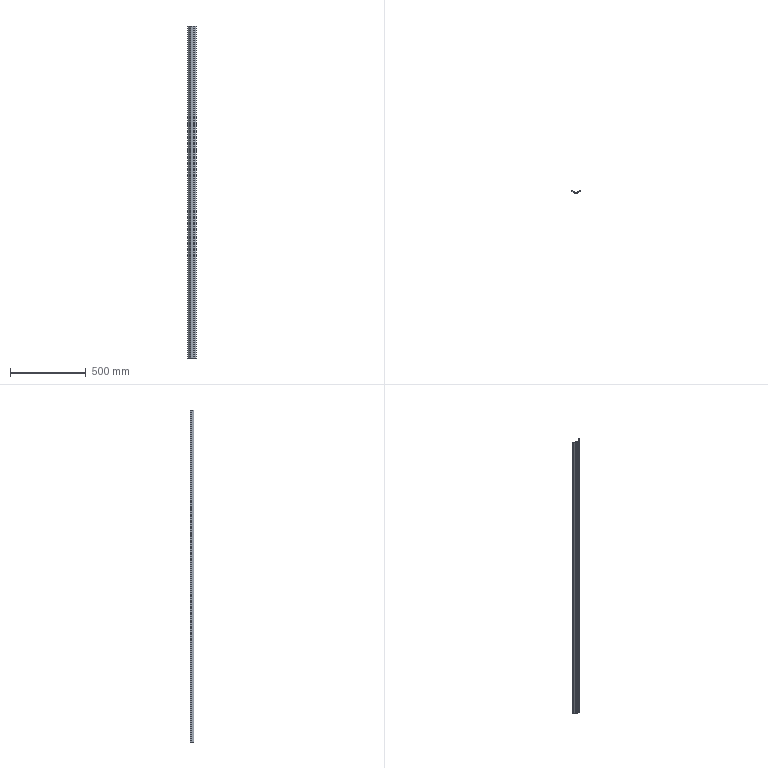Part | 1 solid | 40 faces | box 56.572 x 22.358 x 2185 mm | volume 366285 mm3 | plane 37 | cylinder 3 | commonest cylinder face diameters 1 x2 0.5 x1
STEP:
#1=CARTESIAN_POINT('',(6.75,2.,-1092.5));
#2=VERTEX_POINT('',#1);
#3=CARTESIAN_POINT('',(6.75,5.,-1092.5));
#4=VERTEX_POINT('',#3);
#5=CARTESIAN_POINT('',(6.75,2.,-1092.5));
#6=DIRECTION('',(0.,1.,0.));
#7=VECTOR('',#6,1000.);
#8=LINE('',#5,#7);
#9=EDGE_CURVE('',#2,#4,#8,.T.);
#10=ORIENTED_EDGE('',*,*,#9,.T.);
#11=CARTESIAN_POINT('',(6.75,5.,1092.5));
#12=VERTEX_POINT('',#11);
#13=CARTESIAN_POINT('',(6.75,5.,1092.5));
#14=DIRECTION('',(0.,0.,-1.));
#15=VECTOR('',#14,1000.);
#16=LINE('',#13,#15);
#17=EDGE_CURVE('',#12,#4,#16,.T.);
#18=ORIENTED_EDGE('',*,*,#17,.F.);
#19=CARTESIAN_POINT('',(6.75,2.,1092.5));
#20=VERTEX_POINT('',#19);
#21=CARTESIAN_POINT('',(6.75,2.,1092.5));
#22=DIRECTION('',(0.,1.,0.));
#23=VECTOR('',#22,1000.);
#24=LINE('',#21,#23);
#25=EDGE_CURVE('',#20,#12,#24,.T.);
#26=ORIENTED_EDGE('',*,*,#25,.F.);
#27=CARTESIAN_POINT('',(6.75,2.,1092.5));
#28=DIRECTION('',(0.,0.,-1.));
#29=VECTOR('',#28,1000.);
#30=LINE('',#27,#29);
#31=EDGE_CURVE('',#20,#2,#30,.T.);
#32=ORIENTED_EDGE('',*,*,#31,.T.);
#33=EDGE_LOOP('',(#10,#18,#26,#32));
#34=FACE_OUTER_BOUND('',#33,.T.);
#35=CARTESIAN_POINT('',(6.75,2.,1092.5));
#36=DIRECTION('',(-1.,0.,0.));
#37=DIRECTION('',(0.,0.,1.));
#38=AXIS2_PLACEMENT_3D('',#35,#36,#37);
#39=PLANE('',#38);
#40=ADVANCED_FACE('',(#34),#39,.F.);
#41=CARTESIAN_POINT('',(5.25,5.,-1092.5));
#42=VERTEX_POINT('',#41);
#43=CARTESIAN_POINT('',(6.75,5.,-1092.5));
#44=DIRECTION('',(-1.,0.,0.));
#45=VECTOR('',#44,1000.);
#46=LINE('',#43,#45);
#47=EDGE_CURVE('',#4,#42,#46,.T.);
#48=ORIENTED_EDGE('',*,*,#47,.T.);
#49=CARTESIAN_POINT('',(5.25,5.,1092.5));
#50=VERTEX_POINT('',#49);
#51=CARTESIAN_POINT('',(5.25,5.,1092.5));
#52=DIRECTION('',(0.,0.,-1.));
#53=VECTOR('',#52,1000.);
#54=LINE('',#51,#53);
#55=EDGE_CURVE('',#50,#42,#54,.T.);
#56=ORIENTED_EDGE('',*,*,#55,.F.);
#57=CARTESIAN_POINT('',(6.75,5.,1092.5));
#58=DIRECTION('',(-1.,0.,0.));
#59=VECTOR('',#58,1000.);
#60=LINE('',#57,#59);
#61=EDGE_CURVE('',#12,#50,#60,.T.);
#62=ORIENTED_EDGE('',*,*,#61,.F.);
#63=ORIENTED_EDGE('',*,*,#17,.T.);
#64=EDGE_LOOP('',(#48,#56,#62,#63));
#65=FACE_OUTER_BOUND('',#64,.T.);
#66=CARTESIAN_POINT('',(6.75,5.,1092.5));
#67=DIRECTION('',(0.,-1.,0.));
#68=DIRECTION('',(1.,0.,0.));
#69=AXIS2_PLACEMENT_3D('',#66,#67,#68);
#70=PLANE('',#69);
#71=ADVANCED_FACE('',(#65),#70,.F.);
#72=CARTESIAN_POINT('',(5.25,2.,-1092.5));
#73=VERTEX_POINT('',#72);
#74=CARTESIAN_POINT('',(5.25,5.,-1092.5));
#75=DIRECTION('',(0.,-1.,0.));
#76=VECTOR('',#75,1000.);
#77=LINE('',#74,#76);
#78=EDGE_CURVE('',#42,#73,#77,.T.);
#79=ORIENTED_EDGE('',*,*,#78,.T.);
#80=CARTESIAN_POINT('',(5.25,2.,1092.5));
#81=VERTEX_POINT('',#80);
#82=CARTESIAN_POINT('',(5.25,2.,1092.5));
#83=DIRECTION('',(0.,0.,-1.));
#84=VECTOR('',#83,1000.);
#85=LINE('',#82,#84);
#86=EDGE_CURVE('',#81,#73,#85,.T.);
#87=ORIENTED_EDGE('',*,*,#86,.F.);
#88=CARTESIAN_POINT('',(5.25,5.,1092.5));
#89=DIRECTION('',(0.,-1.,0.));
#90=VECTOR('',#89,1000.);
#91=LINE('',#88,#90);
#92=EDGE_CURVE('',#50,#81,#91,.T.);
#93=ORIENTED_EDGE('',*,*,#92,.F.);
#94=ORIENTED_EDGE('',*,*,#55,.T.);
#95=EDGE_LOOP('',(#79,#87,#93,#94));
#96=FACE_OUTER_BOUND('',#95,.T.);
#97=CARTESIAN_POINT('',(5.25,5.,1092.5));
#98=DIRECTION('',(1.,0.,0.));
#99=DIRECTION('',(0.,0.,-1.));
#100=AXIS2_PLACEMENT_3D('',#97,#98,#99);
#101=PLANE('',#100);
#102=ADVANCED_FACE('',(#96),#101,.F.);
#103=CARTESIAN_POINT('',(0.25,2.,-1092.5));
#104=VERTEX_POINT('',#103);
#105=CARTESIAN_POINT('',(5.25,2.,-1092.5));
#106=DIRECTION('',(-1.,0.,0.));
#107=VECTOR('',#106,1000.);
#108=LINE('',#105,#107);
#109=EDGE_CURVE('',#73,#104,#108,.T.);
#110=ORIENTED_EDGE('',*,*,#109,.T.);
#111=CARTESIAN_POINT('',(0.25,2.,1092.5));
#112=VERTEX_POINT('',#111);
#113=CARTESIAN_POINT('',(0.25,2.,1092.5));
#114=DIRECTION('',(0.,0.,-1.));
#115=VECTOR('',#114,1000.);
#116=LINE('',#113,#115);
#117=EDGE_CURVE('',#112,#104,#116,.T.);
#118=ORIENTED_EDGE('',*,*,#117,.F.);
#119=CARTESIAN_POINT('',(5.25,2.,1092.5));
#120=DIRECTION('',(-1.,0.,0.));
#121=VECTOR('',#120,1000.);
#122=LINE('',#119,#121);
#123=EDGE_CURVE('',#81,#112,#122,.T.);
#124=ORIENTED_EDGE('',*,*,#123,.F.);
#125=ORIENTED_EDGE('',*,*,#86,.T.);
#126=EDGE_LOOP('',(#110,#118,#124,#125));
#127=FACE_OUTER_BOUND('',#126,.T.);
#128=CARTESIAN_POINT('',(5.25,2.,1092.5));
#129=DIRECTION('',(0.,-1.,0.));
#130=DIRECTION('',(0.,0.,-1.));
#131=AXIS2_PLACEMENT_3D('',#128,#129,#130);
#132=PLANE('',#131);
#133=ADVANCED_FACE('',(#127),#132,.F.);
#134=CARTESIAN_POINT('',(-0.25,2.,-1092.5));
#135=VERTEX_POINT('',#134);
#136=CARTESIAN_POINT('',(0.,2.,-1092.5));
#137=DIRECTION('',(0.,0.,-1.));
#138=DIRECTION('',(1.,0.,0.));
#139=AXIS2_PLACEMENT_3D('',#136,#137,#138);
#140=CIRCLE('',#139,0.25);
#141=EDGE_CURVE('',#104,#135,#140,.T.);
#142=ORIENTED_EDGE('',*,*,#141,.T.);
#143=CARTESIAN_POINT('',(-0.25,2.,1092.5));
#144=VERTEX_POINT('',#143);
#145=CARTESIAN_POINT('',(-0.25,2.,1092.5));
#146=DIRECTION('',(0.,0.,-1.));
#147=VECTOR('',#146,1000.);
#148=LINE('',#145,#147);
#149=EDGE_CURVE('',#144,#135,#148,.T.);
#150=ORIENTED_EDGE('',*,*,#149,.F.);
#151=CARTESIAN_POINT('',(0.,2.,1092.5));
#152=DIRECTION('',(0.,0.,-1.));
#153=DIRECTION('',(1.,0.,0.));
#154=AXIS2_PLACEMENT_3D('',#151,#152,#153);
#155=CIRCLE('',#154,0.25);
#156=EDGE_CURVE('',#112,#144,#155,.T.);
#157=ORIENTED_EDGE('',*,*,#156,.F.);
#158=ORIENTED_EDGE('',*,*,#117,.T.);
#159=EDGE_LOOP('',(#142,#150,#157,#158));
#160=FACE_OUTER_BOUND('',#159,.T.);
#161=CARTESIAN_POINT('',(0.,2.,1092.5));
#162=DIRECTION('',(0.,0.,-1.));
#163=DIRECTION('',(-1.,0.,0.));
#164=AXIS2_PLACEMENT_3D('',#161,#162,#163);
#165=CYLINDRICAL_SURFACE('',#164,0.25);
#166=ADVANCED_FACE('',(#160),#165,.F.);
#167=CARTESIAN_POINT('',(-5.25,2.,-1092.5));
#168=VERTEX_POINT('',#167);
#169=CARTESIAN_POINT('',(-0.25,2.,-1092.5));
#170=DIRECTION('',(-1.,0.,0.));
#171=VECTOR('',#170,1000.);
#172=LINE('',#169,#171);
#173=EDGE_CURVE('',#135,#168,#172,.T.);
#174=ORIENTED_EDGE('',*,*,#173,.T.);
#175=CARTESIAN_POINT('',(-5.25,2.,1092.5));
#176=VERTEX_POINT('',#175);
#177=CARTESIAN_POINT('',(-5.25,2.,1092.5));
#178=DIRECTION('',(0.,0.,-1.));
#179=VECTOR('',#178,1000.);
#180=LINE('',#177,#179);
#181=EDGE_CURVE('',#176,#168,#180,.T.);
#182=ORIENTED_EDGE('',*,*,#181,.F.);
#183=CARTESIAN_POINT('',(-0.25,2.,1092.5));
#184=DIRECTION('',(-1.,0.,0.));
#185=VECTOR('',#184,1000.);
#186=LINE('',#183,#185);
#187=EDGE_CURVE('',#144,#176,#186,.T.);
#188=ORIENTED_EDGE('',*,*,#187,.F.);
#189=ORIENTED_EDGE('',*,*,#149,.T.);
#190=EDGE_LOOP('',(#174,#182,#188,#189));
#191=FACE_OUTER_BOUND('',#190,.T.);
#192=CARTESIAN_POINT('',(-0.25,2.,1092.5));
#193=DIRECTION('',(0.,-1.,0.));
#194=DIRECTION('',(1.,0.,0.));
#195=AXIS2_PLACEMENT_3D('',#192,#193,#194);
#196=PLANE('',#195);
#197=ADVANCED_FACE('',(#191),#196,.F.);
#198=CARTESIAN_POINT('',(-5.25,5.,-1092.5));
#199=VERTEX_POINT('',#198);
#200=CARTESIAN_POINT('',(-5.25,2.,-1092.5));
#201=DIRECTION('',(0.,1.,0.));
#202=VECTOR('',#201,1000.);
#203=LINE('',#200,#202);
#204=EDGE_CURVE('',#168,#199,#203,.T.);
#205=ORIENTED_EDGE('',*,*,#204,.T.);
#206=CARTESIAN_POINT('',(-5.25,5.,1092.5));
#207=VERTEX_POINT('',#206);
#208=CARTESIAN_POINT('',(-5.25,5.,1092.5));
#209=DIRECTION('',(0.,0.,-1.));
#210=VECTOR('',#209,1000.);
#211=LINE('',#208,#210);
#212=EDGE_CURVE('',#207,#199,#211,.T.);
#213=ORIENTED_EDGE('',*,*,#212,.F.);
#214=CARTESIAN_POINT('',(-5.25,2.,1092.5));
#215=DIRECTION('',(0.,1.,0.));
#216=VECTOR('',#215,1000.);
#217=LINE('',#214,#216);
#218=EDGE_CURVE('',#176,#207,#217,.T.);
#219=ORIENTED_EDGE('',*,*,#218,.F.);
#220=ORIENTED_EDGE('',*,*,#181,.T.);
#221=EDGE_LOOP('',(#205,#213,#219,#220));
#222=FACE_OUTER_BOUND('',#221,.T.);
#223=CARTESIAN_POINT('',(-5.25,2.,1092.5));
#224=DIRECTION('',(-1.,0.,0.));
#225=DIRECTION('',(0.,0.,1.));
#226=AXIS2_PLACEMENT_3D('',#223,#224,#225);
#227=PLANE('',#226);
#228=ADVANCED_FACE('',(#222),#227,.F.);
#229=CARTESIAN_POINT('',(-6.75,5.,-1092.5));
#230=VERTEX_POINT('',#229);
#231=CARTESIAN_POINT('',(-5.25,5.,-1092.5));
#232=DIRECTION('',(-1.,0.,0.));
#233=VECTOR('',#232,1000.);
#234=LINE('',#231,#233);
#235=EDGE_CURVE('',#199,#230,#234,.T.);
#236=ORIENTED_EDGE('',*,*,#235,.T.);
#237=CARTESIAN_POINT('',(-6.75,5.,1092.5));
#238=VERTEX_POINT('',#237);
#239=CARTESIAN_POINT('',(-6.75,5.,1092.5));
#240=DIRECTION('',(0.,0.,-1.));
#241=VECTOR('',#240,1000.);
#242=LINE('',#239,#241);
#243=EDGE_CURVE('',#238,#230,#242,.T.);
#244=ORIENTED_EDGE('',*,*,#243,.F.);
#245=CARTESIAN_POINT('',(-5.25,5.,1092.5));
#246=DIRECTION('',(-1.,0.,0.));
#247=VECTOR('',#246,1000.);
#248=LINE('',#245,#247);
#249=EDGE_CURVE('',#207,#238,#248,.T.);
#250=ORIENTED_EDGE('',*,*,#249,.F.);
#251=ORIENTED_EDGE('',*,*,#212,.T.);
#252=EDGE_LOOP('',(#236,#244,#250,#251));
#253=FACE_OUTER_BOUND('',#252,.T.);
#254=CARTESIAN_POINT('',(-5.25,5.,1092.5));
#255=DIRECTION('',(0.,-1.,0.));
#256=DIRECTION('',(1.,0.,0.));
#257=AXIS2_PLACEMENT_3D('',#254,#255,#256);
#258=PLANE('',#257);
#259=ADVANCED_FACE('',(#253),#258,.F.);
#260=CARTESIAN_POINT('',(-6.75,2.,-1092.5));
#261=VERTEX_POINT('',#260);
#262=CARTESIAN_POINT('',(-6.75,5.,-1092.5));
#263=DIRECTION('',(0.,-1.,0.));
#264=VECTOR('',#263,1000.);
#265=LINE('',#262,#264);
#266=EDGE_CURVE('',#230,#261,#265,.T.);
#267=ORIENTED_EDGE('',*,*,#266,.T.);
#268=CARTESIAN_POINT('',(-6.75,2.,1092.5));
#269=VERTEX_POINT('',#268);
#270=CARTESIAN_POINT('',(-6.75,2.,1092.5));
#271=DIRECTION('',(0.,0.,-1.));
#272=VECTOR('',#271,1000.);
#273=LINE('',#270,#272);
#274=EDGE_CURVE('',#269,#261,#273,.T.);
#275=ORIENTED_EDGE('',*,*,#274,.F.);
#276=CARTESIAN_POINT('',(-6.75,5.,1092.5));
#277=DIRECTION('',(0.,-1.,0.));
#278=VECTOR('',#277,1000.);
#279=LINE('',#276,#278);
#280=EDGE_CURVE('',#238,#269,#279,.T.);
#281=ORIENTED_EDGE('',*,*,#280,.F.);
#282=ORIENTED_EDGE('',*,*,#243,.T.);
#283=EDGE_LOOP('',(#267,#275,#281,#282));
#284=FACE_OUTER_BOUND('',#283,.T.);
#285=CARTESIAN_POINT('',(-6.75,5.,1092.5));
#286=DIRECTION('',(1.,0.,0.));
#287=DIRECTION('',(0.,0.,-1.));
#288=AXIS2_PLACEMENT_3D('',#285,#286,#287);
#289=PLANE('',#288);
#290=ADVANCED_FACE('',(#284),#289,.F.);
#291=CARTESIAN_POINT('',(-8.635,2.,-1092.5));
#292=VERTEX_POINT('',#291);
#293=CARTESIAN_POINT('',(-6.75,2.,-1092.5));
#294=DIRECTION('',(-1.,0.,0.));
#295=VECTOR('',#294,1000.);
#296=LINE('',#293,#295);
#297=EDGE_CURVE('',#261,#292,#296,.T.);
#298=ORIENTED_EDGE('',*,*,#297,.T.);
#299=CARTESIAN_POINT('',(-8.635,2.,1092.5));
#300=VERTEX_POINT('',#299);
#301=CARTESIAN_POINT('',(-8.635,2.,1092.5));
#302=DIRECTION('',(0.,0.,-1.));
#303=VECTOR('',#302,1000.);
#304=LINE('',#301,#303);
#305=EDGE_CURVE('',#300,#292,#304,.T.);
#306=ORIENTED_EDGE('',*,*,#305,.F.);
#307=CARTESIAN_POINT('',(-6.75,2.,1092.5));
#308=DIRECTION('',(-1.,0.,0.));
#309=VECTOR('',#308,1000.);
#310=LINE('',#307,#309);
#311=EDGE_CURVE('',#269,#300,#310,.T.);
#312=ORIENTED_EDGE('',*,*,#311,.F.);
#313=ORIENTED_EDGE('',*,*,#274,.T.);
#314=EDGE_LOOP('',(#298,#306,#312,#313));
#315=FACE_OUTER_BOUND('',#314,.T.);
#316=CARTESIAN_POINT('',(-6.75,2.,1092.5));
#317=DIRECTION('',(0.,-1.,0.));
#318=DIRECTION('',(1.,0.,0.));
#319=AXIS2_PLACEMENT_3D('',#316,#317,#318);
#320=PLANE('',#319);
#321=ADVANCED_FACE('',(#315),#320,.F.);
#322=CARTESIAN_POINT('',(-11.75,5.119,-1092.5));
#323=VERTEX_POINT('',#322);
#324=CARTESIAN_POINT('',(-8.635,2.,-1092.5));
#325=DIRECTION('',(-0.7067,0.7076,0.));
#326=VECTOR('',#325,1000.);
#327=LINE('',#324,#326);
#328=EDGE_CURVE('',#292,#323,#327,.T.);
#329=ORIENTED_EDGE('',*,*,#328,.T.);
#330=CARTESIAN_POINT('',(-11.75,5.119,1092.5));
#331=VERTEX_POINT('',#330);
#332=CARTESIAN_POINT('',(-11.75,5.119,1092.5));
#333=DIRECTION('',(0.,0.,-1.));
#334=VECTOR('',#333,1000.);
#335=LINE('',#332,#334);
#336=EDGE_CURVE('',#331,#323,#335,.T.);
#337=ORIENTED_EDGE('',*,*,#336,.F.);
#338=CARTESIAN_POINT('',(-8.635,2.,1092.5));
#339=DIRECTION('',(-0.7067,0.7076,0.));
#340=VECTOR('',#339,1000.);
#341=LINE('',#338,#340);
#342=EDGE_CURVE('',#300,#331,#341,.T.);
#343=ORIENTED_EDGE('',*,*,#342,.F.);
#344=ORIENTED_EDGE('',*,*,#305,.T.);
#345=EDGE_LOOP('',(#329,#337,#343,#344));
#346=FACE_OUTER_BOUND('',#345,.T.);
#347=CARTESIAN_POINT('',(-8.635,2.,1092.5));
#348=DIRECTION('',(-0.7076,-0.7067,0.));
#349=DIRECTION('',(0.7067,-0.7076,0.));
#350=AXIS2_PLACEMENT_3D('',#347,#348,#349);
#351=PLANE('',#350);
#352=ADVANCED_FACE('',(#346),#351,.F.);
#353=CARTESIAN_POINT('',(-11.75,8.887,-1092.5));
#354=VERTEX_POINT('',#353);
#355=CARTESIAN_POINT('',(-11.75,5.119,-1092.5));
#356=DIRECTION('',(0.,1.,0.));
#357=VECTOR('',#356,1000.);
#358=LINE('',#355,#357);
#359=EDGE_CURVE('',#323,#354,#358,.T.);
#360=ORIENTED_EDGE('',*,*,#359,.T.);
#361=CARTESIAN_POINT('',(-11.75,8.887,1092.5));
#362=VERTEX_POINT('',#361);
#363=CARTESIAN_POINT('',(-11.75,8.887,1092.5));
#364=DIRECTION('',(0.,0.,-1.));
#365=VECTOR('',#364,1000.);
#366=LINE('',#363,#365);
#367=EDGE_CURVE('',#362,#354,#366,.T.);
#368=ORIENTED_EDGE('',*,*,#367,.F.);
#369=CARTESIAN_POINT('',(-11.75,5.119,1092.5));
#370=DIRECTION('',(0.,1.,0.));
#371=VECTOR('',#370,1000.);
#372=LINE('',#369,#371);
#373=EDGE_CURVE('',#331,#362,#372,.T.);
#374=ORIENTED_EDGE('',*,*,#373,.F.);
#375=ORIENTED_EDGE('',*,*,#336,.T.);
#376=EDGE_LOOP('',(#360,#368,#374,#375));
#377=FACE_OUTER_BOUND('',#376,.T.);
#378=CARTESIAN_POINT('',(-11.75,5.119,1092.5));
#379=DIRECTION('',(-1.,0.,0.));
#380=DIRECTION('',(0.,0.,1.));
#381=AXIS2_PLACEMENT_3D('',#378,#379,#380);
#382=PLANE('',#381);
#383=ADVANCED_FACE('',(#377),#382,.F.);
#384=CARTESIAN_POINT('',(-12.25,9.387,-1092.5));
#385=VERTEX_POINT('',#384);
#386=CARTESIAN_POINT('',(-11.75,8.887,-1092.5));
#387=DIRECTION('',(-0.7071,0.7071,0.));
#388=VECTOR('',#387,1000.);
#389=LINE('',#386,#388);
#390=EDGE_CURVE('',#354,#385,#389,.T.);
#391=ORIENTED_EDGE('',*,*,#390,.T.);
#392=CARTESIAN_POINT('',(-12.25,9.387,1092.5));
#393=VERTEX_POINT('',#392);
#394=CARTESIAN_POINT('',(-12.25,9.387,1092.5));
#395=DIRECTION('',(0.,0.,-1.));
#396=VECTOR('',#395,1000.);
#397=LINE('',#394,#396);
#398=EDGE_CURVE('',#393,#385,#397,.T.);
#399=ORIENTED_EDGE('',*,*,#398,.F.);
#400=CARTESIAN_POINT('',(-11.75,8.887,1092.5));
#401=DIRECTION('',(-0.7071,0.7071,0.));
#402=VECTOR('',#401,1000.);
#403=LINE('',#400,#402);
#404=EDGE_CURVE('',#362,#393,#403,.T.);
#405=ORIENTED_EDGE('',*,*,#404,.F.);
#406=ORIENTED_EDGE('',*,*,#367,.T.);
#407=EDGE_LOOP('',(#391,#399,#405,#406));
#408=FACE_OUTER_BOUND('',#407,.T.);
#409=CARTESIAN_POINT('',(-11.75,8.887,1092.5));
#410=DIRECTION('',(-0.7071,-0.7071,0.));
#411=DIRECTION('',(0.7071,-0.7071,0.));
#412=AXIS2_PLACEMENT_3D('',#409,#410,#411);
#413=PLANE('',#412);
#414=ADVANCED_FACE('',(#408),#413,.F.);
#415=CARTESIAN_POINT('',(-12.75,9.387,-1092.5));
#416=VERTEX_POINT('',#415);
#417=CARTESIAN_POINT('',(-12.25,9.387,-1092.5));
#418=DIRECTION('',(-1.,0.,0.));
#419=VECTOR('',#418,1000.);
#420=LINE('',#417,#419);
#421=EDGE_CURVE('',#385,#416,#420,.T.);
#422=ORIENTED_EDGE('',*,*,#421,.T.);
#423=CARTESIAN_POINT('',(-12.75,9.387,1092.5));
#424=VERTEX_POINT('',#423);
#425=CARTESIAN_POINT('',(-12.75,9.387,1092.5));
#426=DIRECTION('',(0.,0.,-1.));
#427=VECTOR('',#426,1000.);
#428=LINE('',#425,#427);
#429=EDGE_CURVE('',#424,#416,#428,.T.);
#430=ORIENTED_EDGE('',*,*,#429,.F.);
#431=CARTESIAN_POINT('',(-12.25,9.387,1092.5));
#432=DIRECTION('',(-1.,0.,0.));
#433=VECTOR('',#432,1000.);
#434=LINE('',#431,#433);
#435=EDGE_CURVE('',#393,#424,#434,.T.);
#436=ORIENTED_EDGE('',*,*,#435,.F.);
#437=ORIENTED_EDGE('',*,*,#398,.T.);
#438=EDGE_LOOP('',(#422,#430,#436,#437));
#439=FACE_OUTER_BOUND('',#438,.T.);
#440=CARTESIAN_POINT('',(-12.25,9.387,1092.5));
#441=DIRECTION('',(0.,-1.,0.));
#442=DIRECTION('',(0.,0.,-1.));
#443=AXIS2_PLACEMENT_3D('',#440,#441,#442);
#444=PLANE('',#443);
#445=ADVANCED_FACE('',(#439),#444,.F.);
#446=CARTESIAN_POINT('',(-12.75,7.328,-1092.5));
#447=VERTEX_POINT('',#446);
#448=CARTESIAN_POINT('',(-12.75,9.387,-1092.5));
#449=DIRECTION('',(0.,-1.,0.));
#450=VECTOR('',#449,1000.);
#451=LINE('',#448,#450);
#452=EDGE_CURVE('',#416,#447,#451,.T.);
#453=ORIENTED_EDGE('',*,*,#452,.T.);
#454=CARTESIAN_POINT('',(-12.75,7.328,1092.5));
#455=VERTEX_POINT('',#454);
#456=CARTESIAN_POINT('',(-12.75,7.328,1092.5));
#457=DIRECTION('',(0.,0.,-1.));
#458=VECTOR('',#457,1000.);
#459=LINE('',#456,#458);
#460=EDGE_CURVE('',#455,#447,#459,.T.);
#461=ORIENTED_EDGE('',*,*,#460,.F.);
#462=CARTESIAN_POINT('',(-12.75,9.387,1092.5));
#463=DIRECTION('',(0.,-1.,0.));
#464=VECTOR('',#463,1000.);
#465=LINE('',#462,#464);
#466=EDGE_CURVE('',#424,#455,#465,.T.);
#467=ORIENTED_EDGE('',*,*,#466,.F.);
#468=ORIENTED_EDGE('',*,*,#429,.T.);
#469=EDGE_LOOP('',(#453,#461,#467,#468));
#470=FACE_OUTER_BOUND('',#469,.T.);
#471=CARTESIAN_POINT('',(-12.75,9.387,1092.5));
#472=DIRECTION('',(1.,0.,0.));
#473=DIRECTION('',(0.,0.,-1.));
#474=AXIS2_PLACEMENT_3D('',#471,#472,#473);
#475=PLANE('',#474);
#476=ADVANCED_FACE('',(#470),#475,.F.);
#477=CARTESIAN_POINT('',(-13.604,6.975,-1092.5));
#478=VERTEX_POINT('',#477);
#479=CARTESIAN_POINT('',(-13.25,7.328,-1092.5));
#480=DIRECTION('',(0.,0.,-1.));
#481=DIRECTION('',(1.,0.,0.));
#482=AXIS2_PLACEMENT_3D('',#479,#480,#481);
#483=CIRCLE('',#482,0.5);
#484=EDGE_CURVE('',#447,#478,#483,.T.);
#485=ORIENTED_EDGE('',*,*,#484,.T.);
#486=CARTESIAN_POINT('',(-13.604,6.975,1092.5));
#487=VERTEX_POINT('',#486);
#488=CARTESIAN_POINT('',(-13.604,6.975,1092.5));
#489=DIRECTION('',(0.,0.,-1.));
#490=VECTOR('',#489,1000.);
#491=LINE('',#488,#490);
#492=EDGE_CURVE('',#487,#478,#491,.T.);
#493=ORIENTED_EDGE('',*,*,#492,.F.);
#494=CARTESIAN_POINT('',(-13.25,7.328,1092.5));
#495=DIRECTION('',(0.,0.,-1.));
#496=DIRECTION('',(1.,0.,0.));
#497=AXIS2_PLACEMENT_3D('',#494,#495,#496);
#498=CIRCLE('',#497,0.5);
#499=EDGE_CURVE('',#455,#487,#498,.T.);
#500=ORIENTED_EDGE('',*,*,#499,.F.);
#501=ORIENTED_EDGE('',*,*,#460,.T.);
#502=EDGE_LOOP('',(#485,#493,#500,#501));
#503=FACE_OUTER_BOUND('',#502,.T.);
#504=CARTESIAN_POINT('',(-13.25,7.328,1092.5));
#505=DIRECTION('',(0.,0.,-1.));
#506=DIRECTION('',(-1.,0.,0.));
#507=AXIS2_PLACEMENT_3D('',#504,#505,#506);
#508=CYLINDRICAL_SURFACE('',#507,0.5);
#509=ADVANCED_FACE('',(#503),#508,.F.);
#510=CARTESIAN_POINT('',(-23.891,17.282,-1092.5));
#511=VERTEX_POINT('',#510);
#512=CARTESIAN_POINT('',(-13.604,6.975,-1092.5));
#513=DIRECTION('',(-0.7064,0.7078,0.));
#514=VECTOR('',#513,1000.);
#515=LINE('',#512,#514);
#516=EDGE_CURVE('',#478,#511,#515,.T.);
#517=ORIENTED_EDGE('',*,*,#516,.T.);
#518=CARTESIAN_POINT('',(-23.891,17.282,1092.5));
#519=VERTEX_POINT('',#518);
#520=CARTESIAN_POINT('',(-23.891,17.282,1092.5));
#521=DIRECTION('',(0.,0.,-1.));
#522=VECTOR('',#521,1000.);
#523=LINE('',#520,#522);
#524=EDGE_CURVE('',#519,#511,#523,.T.);
#525=ORIENTED_EDGE('',*,*,#524,.F.);
#526=CARTESIAN_POINT('',(-13.604,6.975,1092.5));
#527=DIRECTION('',(-0.7064,0.7078,0.));
#528=VECTOR('',#527,1000.);
#529=LINE('',#526,#528);
#530=EDGE_CURVE('',#487,#519,#529,.T.);
#531=ORIENTED_EDGE('',*,*,#530,.F.);
#532=ORIENTED_EDGE('',*,*,#492,.T.);
#533=EDGE_LOOP('',(#517,#525,#531,#532));
#534=FACE_OUTER_BOUND('',#533,.T.);
#535=CARTESIAN_POINT('',(-13.604,6.975,1092.5));
#536=DIRECTION('',(-0.7078,-0.7064,0.));
#537=DIRECTION('',(0.7064,-0.7078,0.));
#538=AXIS2_PLACEMENT_3D('',#535,#536,#537);
#539=PLANE('',#538);
#540=ADVANCED_FACE('',(#534),#539,.F.);
#541=CARTESIAN_POINT('',(-23.891,19.376,-1092.5));
#542=VERTEX_POINT('',#541);
#543=CARTESIAN_POINT('',(-23.891,17.282,-1092.5));
#544=DIRECTION('',(0.,1.,0.));
#545=VECTOR('',#544,1000.);
#546=LINE('',#543,#545);
#547=EDGE_CURVE('',#511,#542,#546,.T.);
#548=ORIENTED_EDGE('',*,*,#547,.T.);
#549=CARTESIAN_POINT('',(-23.891,19.376,1092.5));
#550=VERTEX_POINT('',#549);
#551=CARTESIAN_POINT('',(-23.891,19.376,1092.5));
#552=DIRECTION('',(0.,0.,-1.));
#553=VECTOR('',#552,1000.);
#554=LINE('',#551,#553);
#555=EDGE_CURVE('',#550,#542,#554,.T.);
#556=ORIENTED_EDGE('',*,*,#555,.F.);
#557=CARTESIAN_POINT('',(-23.891,17.282,1092.5));
#558=DIRECTION('',(0.,1.,0.));
#559=VECTOR('',#558,1000.);
#560=LINE('',#557,#559);
#561=EDGE_CURVE('',#519,#550,#560,.T.);
#562=ORIENTED_EDGE('',*,*,#561,.F.);
#563=ORIENTED_EDGE('',*,*,#524,.T.);
#564=EDGE_LOOP('',(#548,#556,#562,#563));
#565=FACE_OUTER_BOUND('',#564,.T.);
#566=CARTESIAN_POINT('',(-23.891,17.282,1092.5));
#567=DIRECTION('',(-1.,0.,0.));
#568=DIRECTION('',(0.,0.,1.));
#569=AXIS2_PLACEMENT_3D('',#566,#567,#568);
#570=PLANE('',#569);
#571=ADVANCED_FACE('',(#565),#570,.F.);
#572=CARTESIAN_POINT('',(-26.873,22.358,-1092.5));
#573=VERTEX_POINT('',#572);
#574=CARTESIAN_POINT('',(-23.891,19.376,-1092.5));
#575=DIRECTION('',(-0.7071,0.7071,0.));
#576=VECTOR('',#575,1000.);
#577=LINE('',#574,#576);
#578=EDGE_CURVE('',#542,#573,#577,.T.);
#579=ORIENTED_EDGE('',*,*,#578,.T.);
#580=CARTESIAN_POINT('',(-26.873,22.358,1092.5));
#581=VERTEX_POINT('',#580);
#582=CARTESIAN_POINT('',(-26.873,22.358,1092.5));
#583=DIRECTION('',(0.,0.,-1.));
#584=VECTOR('',#583,1000.);
#585=LINE('',#582,#584);
#586=EDGE_CURVE('',#581,#573,#585,.T.);
#587=ORIENTED_EDGE('',*,*,#586,.F.);
#588=CARTESIAN_POINT('',(-23.891,19.376,1092.5));
#589=DIRECTION('',(-0.7071,0.7071,0.));
#590=VECTOR('',#589,1000.);
#591=LINE('',#588,#590);
#592=EDGE_CURVE('',#550,#581,#591,.T.);
#593=ORIENTED_EDGE('',*,*,#592,.F.);
#594=ORIENTED_EDGE('',*,*,#555,.T.);
#595=EDGE_LOOP('',(#579,#587,#593,#594));
#596=FACE_OUTER_BOUND('',#595,.T.);
#597=CARTESIAN_POINT('',(-23.891,19.376,1092.5));
#598=DIRECTION('',(-0.7071,-0.7071,0.));
#599=DIRECTION('',(0.7071,-0.7071,0.));
#600=AXIS2_PLACEMENT_3D('',#597,#598,#599);
#601=PLANE('',#600);
#602=ADVANCED_FACE('',(#596),#601,.F.);
#603=CARTESIAN_POINT('',(-27.58,22.358,-1092.5));
#604=VERTEX_POINT('',#603);
#605=CARTESIAN_POINT('',(-26.873,22.358,-1092.5));
#606=DIRECTION('',(-1.,0.,0.));
#607=VECTOR('',#606,1000.);
#608=LINE('',#605,#607);
#609=EDGE_CURVE('',#573,#604,#608,.T.);
#610=ORIENTED_EDGE('',*,*,#609,.T.);
#611=CARTESIAN_POINT('',(-27.58,22.358,1092.5));
#612=VERTEX_POINT('',#611);
#613=CARTESIAN_POINT('',(-27.58,22.358,1092.5));
#614=DIRECTION('',(0.,0.,-1.));
#615=VECTOR('',#614,1000.);
#616=LINE('',#613,#615);
#617=EDGE_CURVE('',#612,#604,#616,.T.);
#618=ORIENTED_EDGE('',*,*,#617,.F.);
#619=CARTESIAN_POINT('',(-26.873,22.358,1092.5));
#620=DIRECTION('',(-1.,0.,0.));
#621=VECTOR('',#620,1000.);
#622=LINE('',#619,#621);
#623=EDGE_CURVE('',#581,#612,#622,.T.);
#624=ORIENTED_EDGE('',*,*,#623,.F.);
#625=ORIENTED_EDGE('',*,*,#586,.T.);
#626=EDGE_LOOP('',(#610,#618,#624,#625));
#627=FACE_OUTER_BOUND('',#626,.T.);
#628=CARTESIAN_POINT('',(-26.873,22.358,1092.5));
#629=DIRECTION('',(0.,-1.,0.));
#630=DIRECTION('',(0.,0.,-1.));
#631=AXIS2_PLACEMENT_3D('',#628,#629,#630);
#632=PLANE('',#631);
#633=ADVANCED_FACE('',(#627),#632,.F.);
#634=CARTESIAN_POINT('',(-28.284,21.654,-1092.5));
#635=VERTEX_POINT('',#634);
#636=CARTESIAN_POINT('',(-27.58,22.358,-1092.5));
#637=DIRECTION('',(-0.7071,-0.7071,0.));
#638=VECTOR('',#637,1000.);
#639=LINE('',#636,#638);
#640=EDGE_CURVE('',#604,#635,#639,.T.);
#641=ORIENTED_EDGE('',*,*,#640,.T.);
#642=CARTESIAN_POINT('',(-28.284,21.654,1092.5));
#643=VERTEX_POINT('',#642);
#644=CARTESIAN_POINT('',(-28.284,21.654,1092.5));
#645=DIRECTION('',(0.,0.,-1.));
#646=VECTOR('',#645,1000.);
#647=LINE('',#644,#646);
#648=EDGE_CURVE('',#643,#635,#647,.T.);
#649=ORIENTED_EDGE('',*,*,#648,.F.);
#650=CARTESIAN_POINT('',(-27.58,22.358,1092.5));
#651=DIRECTION('',(-0.7071,-0.7071,0.));
#652=VECTOR('',#651,1000.);
#653=LINE('',#650,#652);
#654=EDGE_CURVE('',#612,#643,#653,.T.);
#655=ORIENTED_EDGE('',*,*,#654,.F.);
#656=ORIENTED_EDGE('',*,*,#617,.T.);
#657=EDGE_LOOP('',(#641,#649,#655,#656));
#658=FACE_OUTER_BOUND('',#657,.T.);
#659=CARTESIAN_POINT('',(-27.58,22.358,1092.5));
#660=DIRECTION('',(0.7071,-0.7071,0.));
#661=DIRECTION('',(0.7071,0.7071,0.));
#662=AXIS2_PLACEMENT_3D('',#659,#660,#661);
#663=PLANE('',#662);
#664=ADVANCED_FACE('',(#658),#663,.F.);
#665=CARTESIAN_POINT('',(-28.284,19.103,-1092.5));
#666=VERTEX_POINT('',#665);
#667=CARTESIAN_POINT('',(-28.284,21.654,-1092.5));
#668=DIRECTION('',(0.,-1.,0.));
#669=VECTOR('',#668,1000.);
#670=LINE('',#667,#669);
#671=EDGE_CURVE('',#635,#666,#670,.T.);
#672=ORIENTED_EDGE('',*,*,#671,.T.);
#673=CARTESIAN_POINT('',(-28.284,19.103,1092.5));
#674=VERTEX_POINT('',#673);
#675=CARTESIAN_POINT('',(-28.284,19.103,1092.5));
#676=DIRECTION('',(0.,0.,-1.));
#677=VECTOR('',#676,1000.);
#678=LINE('',#675,#677);
#679=EDGE_CURVE('',#674,#666,#678,.T.);
#680=ORIENTED_EDGE('',*,*,#679,.F.);
#681=CARTESIAN_POINT('',(-28.284,21.654,1092.5));
#682=DIRECTION('',(0.,-1.,0.));
#683=VECTOR('',#682,1000.);
#684=LINE('',#681,#683);
#685=EDGE_CURVE('',#643,#674,#684,.T.);
#686=ORIENTED_EDGE('',*,*,#685,.F.);
#687=ORIENTED_EDGE('',*,*,#648,.T.);
#688=EDGE_LOOP('',(#672,#680,#686,#687));
#689=FACE_OUTER_BOUND('',#688,.T.);
#690=CARTESIAN_POINT('',(-28.284,21.654,1092.5));
#691=DIRECTION('',(1.,0.,0.));
#692=DIRECTION('',(0.,0.,-1.));
#693=AXIS2_PLACEMENT_3D('',#690,#691,#692);
#694=PLANE('',#693);
#695=ADVANCED_FACE('',(#689),#694,.F.);
#696=CARTESIAN_POINT('',(-9.182,0.,-1092.5));
#697=VERTEX_POINT('',#696);
#698=CARTESIAN_POINT('',(-28.284,19.103,-1092.5));
#699=DIRECTION('',(0.7071,-0.7071,0.));
#700=VECTOR('',#699,1000.);
#701=LINE('',#698,#700);
#702=EDGE_CURVE('',#666,#697,#701,.T.);
#703=ORIENTED_EDGE('',*,*,#702,.T.);
#704=CARTESIAN_POINT('',(-9.182,0.,1092.5));
#705=VERTEX_POINT('',#704);
#706=CARTESIAN_POINT('',(-9.182,0.,1092.5));
#707=DIRECTION('',(0.,0.,-1.));
#708=VECTOR('',#707,1000.);
#709=LINE('',#706,#708);
#710=EDGE_CURVE('',#705,#697,#709,.T.);
#711=ORIENTED_EDGE('',*,*,#710,.F.);
#712=CARTESIAN_POINT('',(-28.284,19.103,1092.5));
#713=DIRECTION('',(0.7071,-0.7071,0.));
#714=VECTOR('',#713,1000.);
#715=LINE('',#712,#714);
#716=EDGE_CURVE('',#674,#705,#715,.T.);
#717=ORIENTED_EDGE('',*,*,#716,.F.);
#718=ORIENTED_EDGE('',*,*,#679,.T.);
#719=EDGE_LOOP('',(#703,#711,#717,#718));
#720=FACE_OUTER_BOUND('',#719,.T.);
#721=CARTESIAN_POINT('',(-28.284,19.103,1092.5));
#722=DIRECTION('',(0.7071,0.7071,0.));
#723=DIRECTION('',(-0.7071,0.7071,0.));
#724=AXIS2_PLACEMENT_3D('',#721,#722,#723);
#725=PLANE('',#724);
#726=ADVANCED_FACE('',(#720),#725,.F.);
#727=CARTESIAN_POINT('',(9.182,0.,-1092.5));
#728=VERTEX_POINT('',#727);
#729=CARTESIAN_POINT('',(-9.182,0.,-1092.5));
#730=DIRECTION('',(1.,0.,0.));
#731=VECTOR('',#730,1000.);
#732=LINE('',#729,#731);
#733=EDGE_CURVE('',#697,#728,#732,.T.);
#734=ORIENTED_EDGE('',*,*,#733,.T.);
#735=CARTESIAN_POINT('',(9.182,0.,1092.5));
#736=VERTEX_POINT('',#735);
#737=CARTESIAN_POINT('',(9.182,0.,1092.5));
#738=DIRECTION('',(0.,0.,-1.));
#739=VECTOR('',#738,1000.);
#740=LINE('',#737,#739);
#741=EDGE_CURVE('',#736,#728,#740,.T.);
#742=ORIENTED_EDGE('',*,*,#741,.F.);
#743=CARTESIAN_POINT('',(-9.182,0.,1092.5));
#744=DIRECTION('',(1.,0.,0.));
#745=VECTOR('',#744,1000.);
#746=LINE('',#743,#745);
#747=EDGE_CURVE('',#705,#736,#746,.T.);
#748=ORIENTED_EDGE('',*,*,#747,.F.);
#749=ORIENTED_EDGE('',*,*,#710,.T.);
#750=EDGE_LOOP('',(#734,#742,#748,#749));
#751=FACE_OUTER_BOUND('',#750,.T.);
#752=CARTESIAN_POINT('',(-9.182,0.,1092.5));
#753=DIRECTION('',(0.,1.,0.));
#754=DIRECTION('',(-1.,0.,0.));
#755=AXIS2_PLACEMENT_3D('',#752,#753,#754);
#756=PLANE('',#755);
#757=ADVANCED_FACE('',(#751),#756,.F.);
#758=CARTESIAN_POINT('',(28.287,19.106,-1092.5));
#759=VERTEX_POINT('',#758);
#760=CARTESIAN_POINT('',(9.182,0.,-1092.5));
#761=DIRECTION('',(0.7071,0.7071,0.));
#762=VECTOR('',#761,1000.);
#763=LINE('',#760,#762);
#764=EDGE_CURVE('',#728,#759,#763,.T.);
#765=ORIENTED_EDGE('',*,*,#764,.T.);
#766=CARTESIAN_POINT('',(28.287,19.106,1092.5));
#767=VERTEX_POINT('',#766);
#768=CARTESIAN_POINT('',(28.287,19.106,1092.5));
#769=DIRECTION('',(0.,0.,-1.));
#770=VECTOR('',#769,1000.);
#771=LINE('',#768,#770);
#772=EDGE_CURVE('',#767,#759,#771,.T.);
#773=ORIENTED_EDGE('',*,*,#772,.F.);
#774=CARTESIAN_POINT('',(9.182,0.,1092.5));
#775=DIRECTION('',(0.7071,0.7071,0.));
#776=VECTOR('',#775,1000.);
#777=LINE('',#774,#776);
#778=EDGE_CURVE('',#736,#767,#777,.T.);
#779=ORIENTED_EDGE('',*,*,#778,.F.);
#780=ORIENTED_EDGE('',*,*,#741,.T.);
#781=EDGE_LOOP('',(#765,#773,#779,#780));
#782=FACE_OUTER_BOUND('',#781,.T.);
#783=CARTESIAN_POINT('',(9.182,0.,1092.5));
#784=DIRECTION('',(-0.7071,0.7071,0.));
#785=DIRECTION('',(-0.7071,-0.7071,0.));
#786=AXIS2_PLACEMENT_3D('',#783,#784,#785);
#787=PLANE('',#786);
#788=ADVANCED_FACE('',(#782),#787,.F.);
#789=CARTESIAN_POINT('',(28.287,21.651,-1092.5));
#790=VERTEX_POINT('',#789);
#791=CARTESIAN_POINT('',(28.287,19.106,-1092.5));
#792=DIRECTION('',(0.,1.,0.));
#793=VECTOR('',#792,1000.);
#794=LINE('',#791,#793);
#795=EDGE_CURVE('',#759,#790,#794,.T.);
#796=ORIENTED_EDGE('',*,*,#795,.T.);
#797=CARTESIAN_POINT('',(28.287,21.651,1092.5));
#798=VERTEX_POINT('',#797);
#799=CARTESIAN_POINT('',(28.287,21.651,1092.5));
#800=DIRECTION('',(0.,0.,-1.));
#801=VECTOR('',#800,1000.);
#802=LINE('',#799,#801);
#803=EDGE_CURVE('',#798,#790,#802,.T.);
#804=ORIENTED_EDGE('',*,*,#803,.F.);
#805=CARTESIAN_POINT('',(28.287,19.106,1092.5));
#806=DIRECTION('',(0.,1.,0.));
#807=VECTOR('',#806,1000.);
#808=LINE('',#805,#807);
#809=EDGE_CURVE('',#767,#798,#808,.T.);
#810=ORIENTED_EDGE('',*,*,#809,.F.);
#811=ORIENTED_EDGE('',*,*,#772,.T.);
#812=EDGE_LOOP('',(#796,#804,#810,#811));
#813=FACE_OUTER_BOUND('',#812,.T.);
#814=CARTESIAN_POINT('',(28.287,19.106,1092.5));
#815=DIRECTION('',(-1.,0.,0.));
#816=DIRECTION('',(0.,-1.,0.));
#817=AXIS2_PLACEMENT_3D('',#814,#815,#816);
#818=PLANE('',#817);
#819=ADVANCED_FACE('',(#813),#818,.F.);
#820=CARTESIAN_POINT('',(27.58,22.358,-1092.5));
#821=VERTEX_POINT('',#820);
#822=CARTESIAN_POINT('',(28.287,21.651,-1092.5));
#823=DIRECTION('',(-0.7071,0.7071,0.));
#824=VECTOR('',#823,1000.);
#825=LINE('',#822,#824);
#826=EDGE_CURVE('',#790,#821,#825,.T.);
#827=ORIENTED_EDGE('',*,*,#826,.T.);
#828=CARTESIAN_POINT('',(27.58,22.358,1092.5));
#829=VERTEX_POINT('',#828);
#830=CARTESIAN_POINT('',(27.58,22.358,1092.5));
#831=DIRECTION('',(0.,0.,-1.));
#832=VECTOR('',#831,1000.);
#833=LINE('',#830,#832);
#834=EDGE_CURVE('',#829,#821,#833,.T.);
#835=ORIENTED_EDGE('',*,*,#834,.F.);
#836=CARTESIAN_POINT('',(28.287,21.651,1092.5));
#837=DIRECTION('',(-0.7071,0.7071,0.));
#838=VECTOR('',#837,1000.);
#839=LINE('',#836,#838);
#840=EDGE_CURVE('',#798,#829,#839,.T.);
#841=ORIENTED_EDGE('',*,*,#840,.F.);
#842=ORIENTED_EDGE('',*,*,#803,.T.);
#843=EDGE_LOOP('',(#827,#835,#841,#842));
#844=FACE_OUTER_BOUND('',#843,.T.);
#845=CARTESIAN_POINT('',(28.287,21.651,1092.5));
#846=DIRECTION('',(-0.7071,-0.7071,0.));
#847=DIRECTION('',(0.7071,-0.7071,0.));
#848=AXIS2_PLACEMENT_3D('',#845,#846,#847);
#849=PLANE('',#848);
#850=ADVANCED_FACE('',(#844),#849,.F.);
#851=CARTESIAN_POINT('',(26.873,22.358,-1092.5));
#852=VERTEX_POINT('',#851);
#853=CARTESIAN_POINT('',(27.58,22.358,-1092.5));
#854=DIRECTION('',(-1.,0.,0.));
#855=VECTOR('',#854,1000.);
#856=LINE('',#853,#855);
#857=EDGE_CURVE('',#821,#852,#856,.T.);
#858=ORIENTED_EDGE('',*,*,#857,.T.);
#859=CARTESIAN_POINT('',(26.873,22.358,1092.5));
#860=VERTEX_POINT('',#859);
#861=CARTESIAN_POINT('',(26.873,22.358,1092.5));
#862=DIRECTION('',(0.,0.,-1.));
#863=VECTOR('',#862,1000.);
#864=LINE('',#861,#863);
#865=EDGE_CURVE('',#860,#852,#864,.T.);
#866=ORIENTED_EDGE('',*,*,#865,.F.);
#867=CARTESIAN_POINT('',(27.58,22.358,1092.5));
#868=DIRECTION('',(-1.,0.,0.));
#869=VECTOR('',#868,1000.);
#870=LINE('',#867,#869);
#871=EDGE_CURVE('',#829,#860,#870,.T.);
#872=ORIENTED_EDGE('',*,*,#871,.F.);
#873=ORIENTED_EDGE('',*,*,#834,.T.);
#874=EDGE_LOOP('',(#858,#866,#872,#873));
#875=FACE_OUTER_BOUND('',#874,.T.);
#876=CARTESIAN_POINT('',(27.58,22.358,1092.5));
#877=DIRECTION('',(0.,-1.,0.));
#878=DIRECTION('',(1.,0.,0.));
#879=AXIS2_PLACEMENT_3D('',#876,#877,#878);
#880=PLANE('',#879);
#881=ADVANCED_FACE('',(#875),#880,.F.);
#882=CARTESIAN_POINT('',(23.891,19.376,-1092.5));
#883=VERTEX_POINT('',#882);
#884=CARTESIAN_POINT('',(26.873,22.358,-1092.5));
#885=DIRECTION('',(-0.7071,-0.7071,0.));
#886=VECTOR('',#885,1000.);
#887=LINE('',#884,#886);
#888=EDGE_CURVE('',#852,#883,#887,.T.);
#889=ORIENTED_EDGE('',*,*,#888,.T.);
#890=CARTESIAN_POINT('',(23.891,19.376,1092.5));
#891=VERTEX_POINT('',#890);
#892=CARTESIAN_POINT('',(23.891,19.376,1092.5));
#893=DIRECTION('',(0.,0.,-1.));
#894=VECTOR('',#893,1000.);
#895=LINE('',#892,#894);
#896=EDGE_CURVE('',#891,#883,#895,.T.);
#897=ORIENTED_EDGE('',*,*,#896,.F.);
#898=CARTESIAN_POINT('',(26.873,22.358,1092.5));
#899=DIRECTION('',(-0.7071,-0.7071,0.));
#900=VECTOR('',#899,1000.);
#901=LINE('',#898,#900);
#902=EDGE_CURVE('',#860,#891,#901,.T.);
#903=ORIENTED_EDGE('',*,*,#902,.F.);
#904=ORIENTED_EDGE('',*,*,#865,.T.);
#905=EDGE_LOOP('',(#889,#897,#903,#904));
#906=FACE_OUTER_BOUND('',#905,.T.);
#907=CARTESIAN_POINT('',(26.873,22.358,1092.5));
#908=DIRECTION('',(0.7071,-0.7071,0.));
#909=DIRECTION('',(0.7071,0.7071,0.));
#910=AXIS2_PLACEMENT_3D('',#907,#908,#909);
#911=PLANE('',#910);
#912=ADVANCED_FACE('',(#906),#911,.F.);
#913=CARTESIAN_POINT('',(23.891,17.282,-1092.5));
#914=VERTEX_POINT('',#913);
#915=CARTESIAN_POINT('',(23.891,19.376,-1092.5));
#916=DIRECTION('',(0.,-1.,0.));
#917=VECTOR('',#916,1000.);
#918=LINE('',#915,#917);
#919=EDGE_CURVE('',#883,#914,#918,.T.);
#920=ORIENTED_EDGE('',*,*,#919,.T.);
#921=CARTESIAN_POINT('',(23.891,17.282,1092.5));
#922=VERTEX_POINT('',#921);
#923=CARTESIAN_POINT('',(23.891,17.282,1092.5));
#924=DIRECTION('',(0.,0.,-1.));
#925=VECTOR('',#924,1000.);
#926=LINE('',#923,#925);
#927=EDGE_CURVE('',#922,#914,#926,.T.);
#928=ORIENTED_EDGE('',*,*,#927,.F.);
#929=CARTESIAN_POINT('',(23.891,19.376,1092.5));
#930=DIRECTION('',(0.,-1.,0.));
#931=VECTOR('',#930,1000.);
#932=LINE('',#929,#931);
#933=EDGE_CURVE('',#891,#922,#932,.T.);
#934=ORIENTED_EDGE('',*,*,#933,.F.);
#935=ORIENTED_EDGE('',*,*,#896,.T.);
#936=EDGE_LOOP('',(#920,#928,#934,#935));
#937=FACE_OUTER_BOUND('',#936,.T.);
#938=CARTESIAN_POINT('',(23.891,19.376,1092.5));
#939=DIRECTION('',(1.,0.,0.));
#940=DIRECTION('',(0.,0.,-1.));
#941=AXIS2_PLACEMENT_3D('',#938,#939,#940);
#942=PLANE('',#941);
#943=ADVANCED_FACE('',(#937),#942,.F.);
#944=CARTESIAN_POINT('',(13.604,6.975,-1092.5));
#945=VERTEX_POINT('',#944);
#946=CARTESIAN_POINT('',(23.891,17.282,-1092.5));
#947=DIRECTION('',(-0.7064,-0.7078,0.));
#948=VECTOR('',#947,1000.);
#949=LINE('',#946,#948);
#950=EDGE_CURVE('',#914,#945,#949,.T.);
#951=ORIENTED_EDGE('',*,*,#950,.T.);
#952=CARTESIAN_POINT('',(13.604,6.975,1092.5));
#953=VERTEX_POINT('',#952);
#954=CARTESIAN_POINT('',(13.604,6.975,1092.5));
#955=DIRECTION('',(0.,0.,-1.));
#956=VECTOR('',#955,1000.);
#957=LINE('',#954,#956);
#958=EDGE_CURVE('',#953,#945,#957,.T.);
#959=ORIENTED_EDGE('',*,*,#958,.F.);
#960=CARTESIAN_POINT('',(23.891,17.282,1092.5));
#961=DIRECTION('',(-0.7064,-0.7078,0.));
#962=VECTOR('',#961,1000.);
#963=LINE('',#960,#962);
#964=EDGE_CURVE('',#922,#953,#963,.T.);
#965=ORIENTED_EDGE('',*,*,#964,.F.);
#966=ORIENTED_EDGE('',*,*,#927,.T.);
#967=EDGE_LOOP('',(#951,#959,#965,#966));
#968=FACE_OUTER_BOUND('',#967,.T.);
#969=CARTESIAN_POINT('',(23.891,17.282,1092.5));
#970=DIRECTION('',(0.7078,-0.7064,0.));
#971=DIRECTION('',(0.7064,0.7078,0.));
#972=AXIS2_PLACEMENT_3D('',#969,#970,#971);
#973=PLANE('',#972);
#974=ADVANCED_FACE('',(#968),#973,.F.);
#975=CARTESIAN_POINT('',(12.75,7.328,-1092.5));
#976=VERTEX_POINT('',#975);
#977=CARTESIAN_POINT('',(13.25,7.328,-1092.5));
#978=DIRECTION('',(0.,0.,-1.));
#979=DIRECTION('',(1.,0.,0.));
#980=AXIS2_PLACEMENT_3D('',#977,#978,#979);
#981=CIRCLE('',#980,0.5);
#982=EDGE_CURVE('',#945,#976,#981,.T.);
#983=ORIENTED_EDGE('',*,*,#982,.T.);
#984=CARTESIAN_POINT('',(12.75,7.328,1092.5));
#985=VERTEX_POINT('',#984);
#986=CARTESIAN_POINT('',(12.75,7.328,1092.5));
#987=DIRECTION('',(0.,0.,-1.));
#988=VECTOR('',#987,1000.);
#989=LINE('',#986,#988);
#990=EDGE_CURVE('',#985,#976,#989,.T.);
#991=ORIENTED_EDGE('',*,*,#990,.F.);
#992=CARTESIAN_POINT('',(13.25,7.328,1092.5));
#993=DIRECTION('',(0.,0.,-1.));
#994=DIRECTION('',(1.,0.,0.));
#995=AXIS2_PLACEMENT_3D('',#992,#993,#994);
#996=CIRCLE('',#995,0.5);
#997=EDGE_CURVE('',#953,#985,#996,.T.);
#998=ORIENTED_EDGE('',*,*,#997,.F.);
#999=ORIENTED_EDGE('',*,*,#958,.T.);
#1000=EDGE_LOOP('',(#983,#991,#998,#999));
#1001=FACE_OUTER_BOUND('',#1000,.T.);
#1002=CARTESIAN_POINT('',(13.25,7.328,1092.5));
#1003=DIRECTION('',(0.,0.,-1.));
#1004=DIRECTION('',(-1.,0.,0.));
#1005=AXIS2_PLACEMENT_3D('',#1002,#1003,#1004);
#1006=CYLINDRICAL_SURFACE('',#1005,0.5);
#1007=ADVANCED_FACE('',(#1001),#1006,.F.);
#1008=CARTESIAN_POINT('',(12.75,9.387,-1092.5));
#1009=VERTEX_POINT('',#1008);
#1010=CARTESIAN_POINT('',(12.75,7.328,-1092.5));
#1011=DIRECTION('',(0.,1.,0.));
#1012=VECTOR('',#1011,1000.);
#1013=LINE('',#1010,#1012);
#1014=EDGE_CURVE('',#976,#1009,#1013,.T.);
#1015=ORIENTED_EDGE('',*,*,#1014,.T.);
#1016=CARTESIAN_POINT('',(12.75,9.387,1092.5));
#1017=VERTEX_POINT('',#1016);
#1018=CARTESIAN_POINT('',(12.75,9.387,1092.5));
#1019=DIRECTION('',(0.,0.,-1.));
#1020=VECTOR('',#1019,1000.);
#1021=LINE('',#1018,#1020);
#1022=EDGE_CURVE('',#1017,#1009,#1021,.T.);
#1023=ORIENTED_EDGE('',*,*,#1022,.F.);
#1024=CARTESIAN_POINT('',(12.75,7.328,1092.5));
#1025=DIRECTION('',(0.,1.,0.));
#1026=VECTOR('',#1025,1000.);
#1027=LINE('',#1024,#1026);
#1028=EDGE_CURVE('',#985,#1017,#1027,.T.);
#1029=ORIENTED_EDGE('',*,*,#1028,.F.);
#1030=ORIENTED_EDGE('',*,*,#990,.T.);
#1031=EDGE_LOOP('',(#1015,#1023,#1029,#1030));
#1032=FACE_OUTER_BOUND('',#1031,.T.);
#1033=CARTESIAN_POINT('',(12.75,7.328,1092.5));
#1034=DIRECTION('',(-1.,0.,0.));
#1035=DIRECTION('',(0.,0.,1.));
#1036=AXIS2_PLACEMENT_3D('',#1033,#1034,#1035);
#1037=PLANE('',#1036);
#1038=ADVANCED_FACE('',(#1032),#1037,.F.);
#1039=CARTESIAN_POINT('',(12.25,9.387,-1092.5));
#1040=VERTEX_POINT('',#1039);
#1041=CARTESIAN_POINT('',(12.75,9.387,-1092.5));
#1042=DIRECTION('',(-1.,0.,0.));
#1043=VECTOR('',#1042,1000.);
#1044=LINE('',#1041,#1043);
#1045=EDGE_CURVE('',#1009,#1040,#1044,.T.);
#1046=ORIENTED_EDGE('',*,*,#1045,.T.);
#1047=CARTESIAN_POINT('',(12.25,9.387,1092.5));
#1048=VERTEX_POINT('',#1047);
#1049=CARTESIAN_POINT('',(12.25,9.387,1092.5));
#1050=DIRECTION('',(0.,0.,-1.));
#1051=VECTOR('',#1050,1000.);
#1052=LINE('',#1049,#1051);
#1053=EDGE_CURVE('',#1048,#1040,#1052,.T.);
#1054=ORIENTED_EDGE('',*,*,#1053,.F.);
#1055=CARTESIAN_POINT('',(12.75,9.387,1092.5));
#1056=DIRECTION('',(-1.,0.,0.));
#1057=VECTOR('',#1056,1000.);
#1058=LINE('',#1055,#1057);
#1059=EDGE_CURVE('',#1017,#1048,#1058,.T.);
#1060=ORIENTED_EDGE('',*,*,#1059,.F.);
#1061=ORIENTED_EDGE('',*,*,#1022,.T.);
#1062=EDGE_LOOP('',(#1046,#1054,#1060,#1061));
#1063=FACE_OUTER_BOUND('',#1062,.T.);
#1064=CARTESIAN_POINT('',(12.75,9.387,1092.5));
#1065=DIRECTION('',(0.,-1.,0.));
#1066=DIRECTION('',(1.,0.,0.));
#1067=AXIS2_PLACEMENT_3D('',#1064,#1065,#1066);
#1068=PLANE('',#1067);
#1069=ADVANCED_FACE('',(#1063),#1068,.F.);
#1070=CARTESIAN_POINT('',(11.75,8.887,-1092.5));
#1071=VERTEX_POINT('',#1070);
#1072=CARTESIAN_POINT('',(12.25,9.387,-1092.5));
#1073=DIRECTION('',(-0.7071,-0.7071,0.));
#1074=VECTOR('',#1073,1000.);
#1075=LINE('',#1072,#1074);
#1076=EDGE_CURVE('',#1040,#1071,#1075,.T.);
#1077=ORIENTED_EDGE('',*,*,#1076,.T.);
#1078=CARTESIAN_POINT('',(11.75,8.887,1092.5));
#1079=VERTEX_POINT('',#1078);
#1080=CARTESIAN_POINT('',(11.75,8.887,1092.5));
#1081=DIRECTION('',(0.,0.,-1.));
#1082=VECTOR('',#1081,1000.);
#1083=LINE('',#1080,#1082);
#1084=EDGE_CURVE('',#1079,#1071,#1083,.T.);
#1085=ORIENTED_EDGE('',*,*,#1084,.F.);
#1086=CARTESIAN_POINT('',(12.25,9.387,1092.5));
#1087=DIRECTION('',(-0.7071,-0.7071,0.));
#1088=VECTOR('',#1087,1000.);
#1089=LINE('',#1086,#1088);
#1090=EDGE_CURVE('',#1048,#1079,#1089,.T.);
#1091=ORIENTED_EDGE('',*,*,#1090,.F.);
#1092=ORIENTED_EDGE('',*,*,#1053,.T.);
#1093=EDGE_LOOP('',(#1077,#1085,#1091,#1092));
#1094=FACE_OUTER_BOUND('',#1093,.T.);
#1095=CARTESIAN_POINT('',(12.25,9.387,1092.5));
#1096=DIRECTION('',(0.7071,-0.7071,0.));
#1097=DIRECTION('',(0.7071,0.7071,0.));
#1098=AXIS2_PLACEMENT_3D('',#1095,#1096,#1097);
#1099=PLANE('',#1098);
#1100=ADVANCED_FACE('',(#1094),#1099,.F.);
#1101=CARTESIAN_POINT('',(11.75,5.119,-1092.5));
#1102=VERTEX_POINT('',#1101);
#1103=CARTESIAN_POINT('',(11.75,8.887,-1092.5));
#1104=DIRECTION('',(0.,-1.,0.));
#1105=VECTOR('',#1104,1000.);
#1106=LINE('',#1103,#1105);
#1107=EDGE_CURVE('',#1071,#1102,#1106,.T.);
#1108=ORIENTED_EDGE('',*,*,#1107,.T.);
#1109=CARTESIAN_POINT('',(11.75,5.119,1092.5));
#1110=VERTEX_POINT('',#1109);
#1111=CARTESIAN_POINT('',(11.75,5.119,1092.5));
#1112=DIRECTION('',(0.,0.,-1.));
#1113=VECTOR('',#1112,1000.);
#1114=LINE('',#1111,#1113);
#1115=EDGE_CURVE('',#1110,#1102,#1114,.T.);
#1116=ORIENTED_EDGE('',*,*,#1115,.F.);
#1117=CARTESIAN_POINT('',(11.75,8.887,1092.5));
#1118=DIRECTION('',(0.,-1.,0.));
#1119=VECTOR('',#1118,1000.);
#1120=LINE('',#1117,#1119);
#1121=EDGE_CURVE('',#1079,#1110,#1120,.T.);
#1122=ORIENTED_EDGE('',*,*,#1121,.F.);
#1123=ORIENTED_EDGE('',*,*,#1084,.T.);
#1124=EDGE_LOOP('',(#1108,#1116,#1122,#1123));
#1125=FACE_OUTER_BOUND('',#1124,.T.);
#1126=CARTESIAN_POINT('',(11.75,8.887,1092.5));
#1127=DIRECTION('',(1.,0.,0.));
#1128=DIRECTION('',(0.,0.,-1.));
#1129=AXIS2_PLACEMENT_3D('',#1126,#1127,#1128);
#1130=PLANE('',#1129);
#1131=ADVANCED_FACE('',(#1125),#1130,.F.);
#1132=CARTESIAN_POINT('',(8.636,2.,-1092.5));
#1133=VERTEX_POINT('',#1132);
#1134=CARTESIAN_POINT('',(11.75,5.119,-1092.5));
#1135=DIRECTION('',(-0.7066,-0.7076,0.));
#1136=VECTOR('',#1135,1000.);
#1137=LINE('',#1134,#1136);
#1138=EDGE_CURVE('',#1102,#1133,#1137,.T.);
#1139=ORIENTED_EDGE('',*,*,#1138,.T.);
#1140=CARTESIAN_POINT('',(8.636,2.,1092.5));
#1141=VERTEX_POINT('',#1140);
#1142=CARTESIAN_POINT('',(8.636,2.,1092.5));
#1143=DIRECTION('',(0.,0.,-1.));
#1144=VECTOR('',#1143,1000.);
#1145=LINE('',#1142,#1144);
#1146=EDGE_CURVE('',#1141,#1133,#1145,.T.);
#1147=ORIENTED_EDGE('',*,*,#1146,.F.);
#1148=CARTESIAN_POINT('',(11.75,5.119,1092.5));
#1149=DIRECTION('',(-0.7066,-0.7076,0.));
#1150=VECTOR('',#1149,1000.);
#1151=LINE('',#1148,#1150);
#1152=EDGE_CURVE('',#1110,#1141,#1151,.T.);
#1153=ORIENTED_EDGE('',*,*,#1152,.F.);
#1154=ORIENTED_EDGE('',*,*,#1115,.T.);
#1155=EDGE_LOOP('',(#1139,#1147,#1153,#1154));
#1156=FACE_OUTER_BOUND('',#1155,.T.);
#1157=CARTESIAN_POINT('',(11.75,5.119,1092.5));
#1158=DIRECTION('',(0.7076,-0.7066,0.));
#1159=DIRECTION('',(0.7066,0.7076,0.));
#1160=AXIS2_PLACEMENT_3D('',#1157,#1158,#1159);
#1161=PLANE('',#1160);
#1162=ADVANCED_FACE('',(#1156),#1161,.F.);
#1163=CARTESIAN_POINT('',(8.636,2.,-1092.5));
#1164=DIRECTION('',(-1.,0.,0.));
#1165=VECTOR('',#1164,1000.);
#1166=LINE('',#1163,#1165);
#1167=EDGE_CURVE('',#1133,#2,#1166,.T.);
#1168=ORIENTED_EDGE('',*,*,#1167,.T.);
#1169=ORIENTED_EDGE('',*,*,#31,.F.);
#1170=CARTESIAN_POINT('',(8.636,2.,1092.5));
#1171=DIRECTION('',(-1.,0.,0.));
#1172=VECTOR('',#1171,1000.);
#1173=LINE('',#1170,#1172);
#1174=EDGE_CURVE('',#1141,#20,#1173,.T.);
#1175=ORIENTED_EDGE('',*,*,#1174,.F.);
#1176=ORIENTED_EDGE('',*,*,#1146,.T.);
#1177=EDGE_LOOP('',(#1168,#1169,#1175,#1176));
#1178=FACE_OUTER_BOUND('',#1177,.T.);
#1179=CARTESIAN_POINT('',(8.636,2.,1092.5));
#1180=DIRECTION('',(0.,-1.,0.));
#1181=DIRECTION('',(0.,0.,-1.));
#1182=AXIS2_PLACEMENT_3D('',#1179,#1180,#1181);
#1183=PLANE('',#1182);
#1184=ADVANCED_FACE('',(#1178),#1183,.F.);
#1185=ORIENTED_EDGE('',*,*,#25,.T.);
#1186=ORIENTED_EDGE('',*,*,#61,.T.);
#1187=ORIENTED_EDGE('',*,*,#92,.T.);
#1188=ORIENTED_EDGE('',*,*,#123,.T.);
#1189=ORIENTED_EDGE('',*,*,#156,.T.);
#1190=ORIENTED_EDGE('',*,*,#187,.T.);
#1191=ORIENTED_EDGE('',*,*,#218,.T.);
#1192=ORIENTED_EDGE('',*,*,#249,.T.);
#1193=ORIENTED_EDGE('',*,*,#280,.T.);
#1194=ORIENTED_EDGE('',*,*,#311,.T.);
#1195=ORIENTED_EDGE('',*,*,#342,.T.);
#1196=ORIENTED_EDGE('',*,*,#373,.T.);
#1197=ORIENTED_EDGE('',*,*,#404,.T.);
#1198=ORIENTED_EDGE('',*,*,#435,.T.);
#1199=ORIENTED_EDGE('',*,*,#466,.T.);
#1200=ORIENTED_EDGE('',*,*,#499,.T.);
#1201=ORIENTED_EDGE('',*,*,#530,.T.);
#1202=ORIENTED_EDGE('',*,*,#561,.T.);
#1203=ORIENTED_EDGE('',*,*,#592,.T.);
#1204=ORIENTED_EDGE('',*,*,#623,.T.);
#1205=ORIENTED_EDGE('',*,*,#654,.T.);
#1206=ORIENTED_EDGE('',*,*,#685,.T.);
#1207=ORIENTED_EDGE('',*,*,#716,.T.);
#1208=ORIENTED_EDGE('',*,*,#747,.T.);
#1209=ORIENTED_EDGE('',*,*,#778,.T.);
#1210=ORIENTED_EDGE('',*,*,#809,.T.);
#1211=ORIENTED_EDGE('',*,*,#840,.T.);
#1212=ORIENTED_EDGE('',*,*,#871,.T.);
#1213=ORIENTED_EDGE('',*,*,#902,.T.);
#1214=ORIENTED_EDGE('',*,*,#933,.T.);
#1215=ORIENTED_EDGE('',*,*,#964,.T.);
#1216=ORIENTED_EDGE('',*,*,#997,.T.);
#1217=ORIENTED_EDGE('',*,*,#1028,.T.);
#1218=ORIENTED_EDGE('',*,*,#1059,.T.);
#1219=ORIENTED_EDGE('',*,*,#1090,.T.);
#1220=ORIENTED_EDGE('',*,*,#1121,.T.);
#1221=ORIENTED_EDGE('',*,*,#1152,.T.);
#1222=ORIENTED_EDGE('',*,*,#1174,.T.);
#1223=EDGE_LOOP('',(#1185,#1186,#1187,#1188,#1189,#1190,#1191,#1192,#1193,#1194,#1195,#1196,#1197,#1198,#1199,#1200,#1201,#1202,#1203,#1204,#1205,#1206,#1207,#1208,#1209,#1210,#1211,#1212,#1213,#1214,#1215,#1216,#1217,#1218,#1219,#1220,#1221,#1222));
#1224=FACE_OUTER_BOUND('',#1223,.T.);
#1225=CARTESIAN_POINT('',(0.,2.,1092.5));
#1226=DIRECTION('',(0.,0.,1.));
#1227=DIRECTION('',(1.,0.,0.));
#1228=AXIS2_PLACEMENT_3D('',#1225,#1226,#1227);
#1229=PLANE('',#1228);
#1230=ADVANCED_FACE('',(#1224),#1229,.T.);
#1231=ORIENTED_EDGE('',*,*,#9,.F.);
#1232=ORIENTED_EDGE('',*,*,#1167,.F.);
#1233=ORIENTED_EDGE('',*,*,#1138,.F.);
#1234=ORIENTED_EDGE('',*,*,#1107,.F.);
#1235=ORIENTED_EDGE('',*,*,#1076,.F.);
#1236=ORIENTED_EDGE('',*,*,#1045,.F.);
#1237=ORIENTED_EDGE('',*,*,#1014,.F.);
#1238=ORIENTED_EDGE('',*,*,#982,.F.);
#1239=ORIENTED_EDGE('',*,*,#950,.F.);
#1240=ORIENTED_EDGE('',*,*,#919,.F.);
#1241=ORIENTED_EDGE('',*,*,#888,.F.);
#1242=ORIENTED_EDGE('',*,*,#857,.F.);
#1243=ORIENTED_EDGE('',*,*,#826,.F.);
#1244=ORIENTED_EDGE('',*,*,#795,.F.);
#1245=ORIENTED_EDGE('',*,*,#764,.F.);
#1246=ORIENTED_EDGE('',*,*,#733,.F.);
#1247=ORIENTED_EDGE('',*,*,#702,.F.);
#1248=ORIENTED_EDGE('',*,*,#671,.F.);
#1249=ORIENTED_EDGE('',*,*,#640,.F.);
#1250=ORIENTED_EDGE('',*,*,#609,.F.);
#1251=ORIENTED_EDGE('',*,*,#578,.F.);
#1252=ORIENTED_EDGE('',*,*,#547,.F.);
#1253=ORIENTED_EDGE('',*,*,#516,.F.);
#1254=ORIENTED_EDGE('',*,*,#484,.F.);
#1255=ORIENTED_EDGE('',*,*,#452,.F.);
#1256=ORIENTED_EDGE('',*,*,#421,.F.);
#1257=ORIENTED_EDGE('',*,*,#390,.F.);
#1258=ORIENTED_EDGE('',*,*,#359,.F.);
#1259=ORIENTED_EDGE('',*,*,#328,.F.);
#1260=ORIENTED_EDGE('',*,*,#297,.F.);
#1261=ORIENTED_EDGE('',*,*,#266,.F.);
#1262=ORIENTED_EDGE('',*,*,#235,.F.);
#1263=ORIENTED_EDGE('',*,*,#204,.F.);
#1264=ORIENTED_EDGE('',*,*,#173,.F.);
#1265=ORIENTED_EDGE('',*,*,#141,.F.);
#1266=ORIENTED_EDGE('',*,*,#109,.F.);
#1267=ORIENTED_EDGE('',*,*,#78,.F.);
#1268=ORIENTED_EDGE('',*,*,#47,.F.);
#1269=EDGE_LOOP('',(#1231,#1232,#1233,#1234,#1235,#1236,#1237,#1238,#1239,#1240,#1241,#1242,#1243,#1244,#1245,#1246,#1247,#1248,#1249,#1250,#1251,#1252,#1253,#1254,#1255,#1256,#1257,#1258,#1259,#1260,#1261,#1262,#1263,#1264,#1265,#1266,#1267,#1268));
#1270=FACE_OUTER_BOUND('',#1269,.T.);
#1271=CARTESIAN_POINT('',(0.,2.,-1092.5));
#1272=DIRECTION('',(0.,0.,1.));
#1273=DIRECTION('',(1.,0.,0.));
#1274=AXIS2_PLACEMENT_3D('',#1271,#1272,#1273);
#1275=PLANE('',#1274);
#1276=ADVANCED_FACE('',(#1270),#1275,.F.);
#1277=CLOSED_SHELL('',(#40,#71,#102,#133,#166,#197,#228,#259,#290,#321,#352,#383,#414,#445,#476,#509,#540,#571,#602,#633,#664,#695,#726,#757,#788,#819,#850,#881,#912,#943,#974,#1007,#1038,#1069,#1100,#1131,#1162,#1184,#1230,#1276));
#1278=MANIFOLD_SOLID_BREP('',#1277);
#1279=CARTESIAN_POINT('',(0.,0.,0.));
#1280=DIRECTION('',(0.,0.,1.));
#1281=DIRECTION('',(1.,0.,0.));
#1282=AXIS2_PLACEMENT_3D('',#1279,#1280,#1281);
#1283=(LENGTH_UNIT()NAMED_UNIT(*)SI_UNIT(.MILLI.,.METRE.));
#1284=UNCERTAINTY_MEASURE_WITH_UNIT(LENGTH_MEASURE(0.00001),#1283,'','');
#1285=(NAMED_UNIT(*)PLANE_ANGLE_UNIT()SI_UNIT($,.RADIAN.));
#1286=(NAMED_UNIT(*)SI_UNIT($,.STERADIAN.)SOLID_ANGLE_UNIT());
#1287=(GEOMETRIC_REPRESENTATION_CONTEXT(3)GLOBAL_UNCERTAINTY_ASSIGNED_CONTEXT((#1284))GLOBAL_UNIT_ASSIGNED_CONTEXT((#1283,#1285,#1286))REPRESENTATION_CONTEXT('',''));
#1288=ADVANCED_BREP_SHAPE_REPRESENTATION('',(#1278,#1282),#1287);